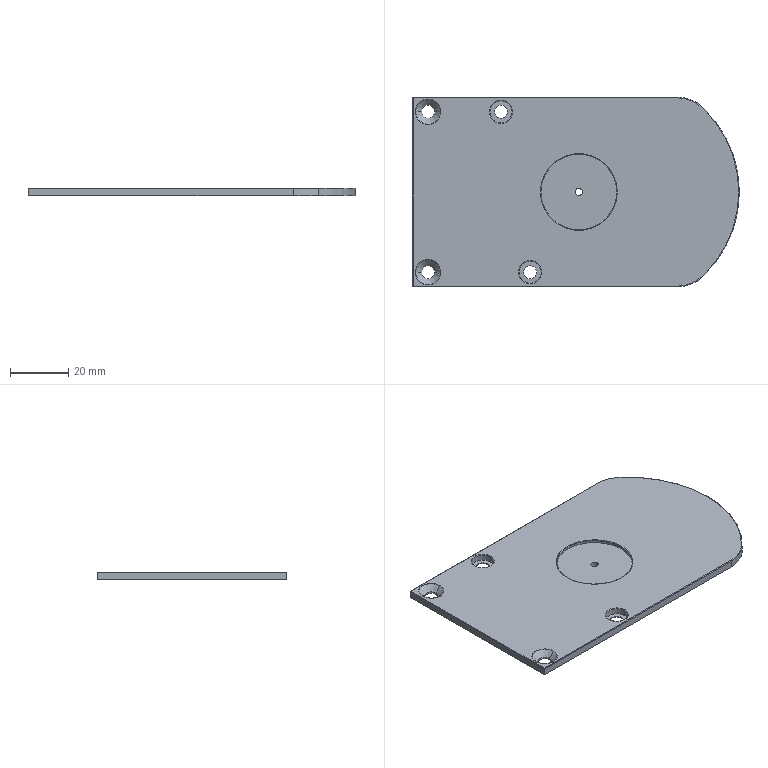Part | STEP file | 1 solid | 47 faces | box 112.05 x 65 x 2.65 mm | volume 17494 mm3 | cylinder 22 | torus 13 | plane 8 | cone 4 | commonest cylinder face diameters 4.5 x8 7.6 x4 0.4 x3 2.5 x2 25.5 x2 26 x2